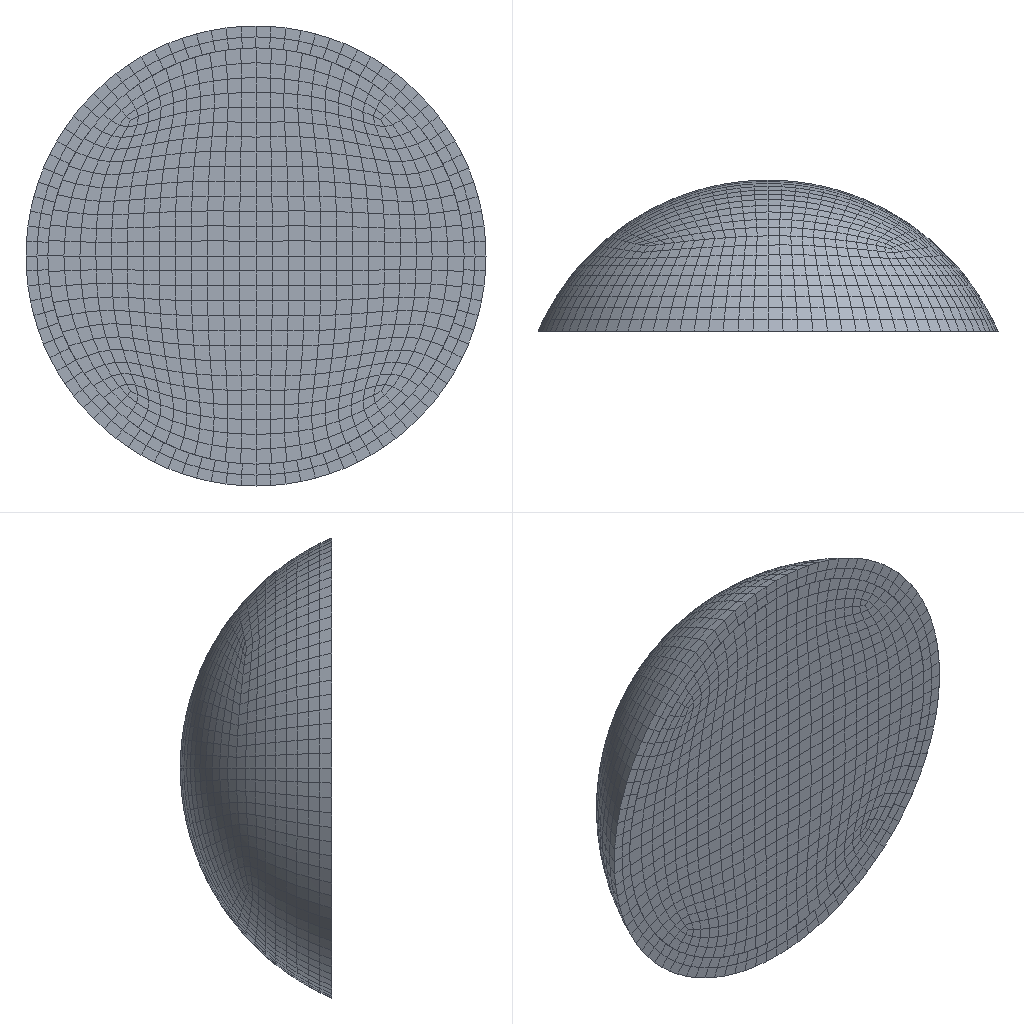Simulation study | abaqus
Set-up summary:
category,name,step,type,value,unit,region
solver,abaqus
solver,version,,,Abaqus/Standard 2020
units,not stated in the deck,,not stated
analysis,deck,,static,static
load_step,Step-1,Step-1,static,nlgeom=True
contact,interactions,,,general=1 pairs=0 ties=0
load_step,requested,,,1
mesh,nodes,,,10810
mesh,elements,,,8352
element_type,C3D8R,,solid,8352
load,load commands in deck,,count,1
bc,support commands in deck,,count,6
material,JITI,,in results
material,MATERIAL-2,,in results
material,MATERIAL-2-COPY,,in results
check,setup vs results,,match,"per instance, exact: element labels, types and connectivity; labels of the nodes the elements use; coordinates not compared"
Abaqus input file, long lists of numbers shortened:
*Heading
** Job name: Job-1 Model name: Model-1
** Generated by: Abaqus/CAE 2020
*Preprint, echo=NO, model=NO, history=NO, contact=NO
**
** PARTS
**
*Part, name=Part-1
*Node
      1,           0.,           0., -0.009499
      2,           0., 0.006,           0.
** (6340 more lines like these left out)
*Element, type=C3D8R
   1,  515,  516, 2283, 2095,   17,   18,  208,  207
   2,  516,  517, 2284, 2283,   18,   19,  209,  208
** (5470 more lines like these left out)
*Node
   6343, 6.44164214e-19, 0.006,           0.
*Nset, nset=Part-1-RefPt_, internal
6343,
*Nset, nset=Set-1, generate
    1,  6342,     1
*Elset, elset=Set-1, generate
    1,  5472,     1
** Section: jiti
*Solid Section, elset=Set-1, material=jiti
,
*End Part
**
*Part, name=mo
*Node
      1,           0., 0.003, 0.007357
      2,           0., 0.003, 0.008609
** (4465 more lines like these left out)
*Element, type=C3D8R
  1,  124,  824, 3248,  594,    1,   19,  548,   66
  2,  824,  130,  709, 3248,   19,    2,   20,  548
** (2878 more lines like these left out)
*Nset, nset=Set-4, generate
    1,  4467,     1
*Elset, elset=Set-4, generate
    1,  2880,     1
*Nset, nset=Set-20
    1,    2,    3,    4,    9,   10,   11,   12,   17,   18,   19,   20,   21,   22,   23,   24
   25,   26,   27,   28,   29,   30,   31,   32,   33,   34,   35,   36,   37,   38,   39,   40
** (170 more lines like these left out)
*Elset, elset=Set-20, generate
  865,  2592,     1
*Nset, nset=Set-21
    1,    2,    3,    4,    5,    6,    7,    8,    9,   10,   11,   12,   13,   14,   15,   16
   19,   20,   21,   22,   23,   24,   25,   26,   27,   28,   29,   30,   31,   32,   33,   34
** (124 more lines like these left out)
*Elset, elset=Set-21
    1,    2,    3,    4,    5,    6,    7,    8,    9,   10,   11,   12,   13,   14,   15,   16
   17,   18,   19,   20,   21,   22,   23,   24,   25,   26,   27,   28,   29,   30,   31,   32
** (70 more lines like these left out)
** Section: mokuai
*Solid Section, elset=Set-21, material=Material-2-Copy
,
** Section: mo
*Solid Section, elset=Set-20, material=Material-2
,
*End Part
**
**
** ASSEMBLY
**
*Assembly, name=Assembly
**
*Instance, name=Part-1-1, part=Part-1
*End Instance
**
*Instance, name=mo-1, part=mo
*End Instance
**
*Nset, nset=Set-3, instance=Part-1-1
 6343,
*Nset, nset=Set-4, instance=mo-1, generate
    1,  4467,     1
*Elset, elset=Set-4, instance=mo-1, generate
    1,  2880,     1
*Nset, nset=Set-5, instance=mo-1, generate
    1,  4467,     1
*Elset, elset=Set-5, instance=mo-1, generate
    1,  2880,     1
*Nset, nset=Set-6, instance=mo-1
 17,
*Nset, nset=Set-7, instance=mo-1
 17,
*Nset, nset=Set-8, instance=mo-1
    5,    6,    7,    8,   13,   14,   15,   16,   17,   18,   67,   68,   69,   70,   71,   72
   73,   74,   75,   76,   77,   78,   79,   80,   81,   82,   83,   84,   85,   86,   87,   88
** (17 more lines like these left out)
*Elset, elset=Set-8, instance=mo-1
  241,  242,  243,  244,  245,  246,  247,  248,  249,  250,  251,  252,  253,  254,  255,  256
  257,  258,  259,  260,  261,  262,  263,  264,  265,  266,  267,  268,  269,  270,  271,  272
** (11 more lines like these left out)
*Nset, nset=Set-9, instance=mo-1, generate
    1,  4467,     1
*Elset, elset=Set-9, instance=mo-1, generate
    1,  2880,     1
*Nset, nset=b_Set-1, instance=Part-1-1, generate
    1,  6342,     1
*Elset, elset=b_Set-1, instance=Part-1-1, generate
    1,  5472,     1
*Nset, nset=_PickedSet7, internal, instance=Part-1-1
 6343,
*Elset, elset=_Surf-1_S1, internal, instance=mo-1, generate
 2737,  2880,     1
*Elset, elset=_Surf-1_S3, internal, instance=mo-1
 1945, 1946, 1947, 1948, 1949, 1950, 1951, 1952, 1953, 1954, 1955, 1956, 1957, 1958, 1959, 1960
 1961, 1962, 1963, 1964, 1965, 1966, 1967, 1968, 1969, 1970, 1971, 1972, 1973, 1974, 1975, 1976
** (21 more lines like these left out)
*Elset, elset=_Surf-1_S4, internal, instance=mo-1
    2,    4,    6,    8,   10,   12,   14,   16,   18,   20,   22,   24,   26,   28,   30,   32
   34,   36,   38,   40,   42,   44,   46,   48,   50,   52,   54,   56,   58,   60,   62,   64
** (21 more lines like these left out)
*Elset, elset=_Surf-1_S5, internal, instance=mo-1
 601, 602, 603, 604, 605, 606, 607, 608, 609, 610, 611, 612, 613, 614, 615, 616
 617, 618, 619, 620, 621, 622, 623, 624, 649, 650, 651, 652, 653, 654, 655, 656
** (7 more lines like these left out)
*Elset, elset=_Surf-1_S2, internal, instance=mo-1
  865,  866,  867,  868,  869,  870,  871,  872,  873,  874,  875,  876,  877,  878,  879,  880
  881,  882,  883,  884,  885,  886,  887,  888,  889,  890,  891,  892,  893,  894,  895,  896
** (25 more lines like these left out)
*Surface, type=ELEMENT, name=Surf-1
_Surf-1_S1, S1
_Surf-1_S3, S3
_Surf-1_S4, S4
_Surf-1_S2, S2
_Surf-1_S5, S5
** Constraint: Constraint-1
*Rigid Body, ref node=_PickedSet7, elset=b_Set-1
*Elset, elset=__Int-1_gcs0_4_S2, internal, instance=Part-1-1
   1,   2,   3,   4,   5,   6,   7,   8,   9,  10,  11,  12,  13,  14,  15,  16
  17,  18,  19,  20,  21,  22,  23,  24,  25,  26,  27,  28,  29,  30,  31,  32
** (13 more lines like these left out)
*Surface, type=ELEMENT, name=_Int-1_gcs0_4, internal
__Int-1_gcs0_4_S2, S2
*Elset, elset=__Int-1_gcs0_5_S4, internal, instance=Part-1-1
 4767, 4770, 4773, 4776, 4779, 4782, 4785, 4788, 4791, 4794, 4797, 4800, 4803, 4806, 4809, 4812
 4815, 4818, 4821, 4824, 4827, 4830, 4833, 4836, 4839, 4842, 4845, 4848, 4851, 4854, 4857, 4860
** (9 more lines like these left out)
*Elset, elset=__Int-1_gcs0_5_S3, internal, instance=Part-1-1
 4945, 4946, 4947, 4948, 4949, 4950, 4951, 4952, 4953, 4954, 4955, 4978, 4979, 4980, 4981, 4982
 4983, 4984, 4985, 4986, 4987, 4988, 5011, 5012, 5013, 5014, 5015, 5016, 5017, 5018, 5019, 5020
** (3 more lines like these left out)
*Surface, type=ELEMENT, name=_Int-1_gcs0_5, internal
__Int-1_gcs0_5_S4, S4
__Int-1_gcs0_5_S3, S3
*Elset, elset=__Int-1_gcs0_10_S3, internal, instance=Part-1-1
 1369, 1370, 1371, 1372, 1373, 1374, 1375, 1376, 1377, 1378, 1399, 1400, 1401, 1402, 1403, 1404
 1405, 1406, 1407, 1408, 1429, 1430, 1431, 1432, 1433, 1434, 1435, 1436, 1437, 1438, 1459, 1460
** (9 more lines like these left out)
*Elset, elset=__Int-1_gcs0_10_S4, internal, instance=Part-1-1, generate
 2211,  2406,     3
*Surface, type=ELEMENT, name=_Int-1_gcs0_10, internal
__Int-1_gcs0_10_S3, S3
__Int-1_gcs0_10_S4, S4
*Elset, elset=__Int-1_gcs0_11_S4, internal, instance=Part-1-1
 2739, 2742, 2745, 2748, 2751, 2754, 2757, 2760, 2763, 2766, 2769, 2772, 2775, 2778, 2781, 2784
 2787, 2790, 2793, 2796, 2799, 2802, 2805, 2808, 2811, 2814, 2817, 2820, 2823, 2826, 2829, 2832
** (9 more lines like these left out)
*Elset, elset=__Int-1_gcs0_11_S3, internal, instance=Part-1-1
 3727, 3728, 3729, 3730, 3731, 3732, 3745, 3746, 3747, 3748, 3749, 3750, 3763, 3764, 3765, 3766
 3767, 3768, 3781, 3782, 3783, 3784, 3785, 3786, 3799, 3800, 3801, 3802, 3803, 3804, 3817, 3818
** (3 more lines like these left out)
*Surface, type=ELEMENT, name=_Int-1_gcs0_11, internal
__Int-1_gcs0_11_S4, S4
__Int-1_gcs0_11_S3, S3
*Elset, elset=__Int-1_gcs0_17_S2, internal, instance=mo-1, generate
  865,  1080,     1
*Surface, type=ELEMENT, name=_Int-1_gcs0_17, internal
__Int-1_gcs0_17_S2, S2
*Elset, elset=__Int-1_gcs0_18_S1, internal, instance=mo-1, generate
 2737,  2880,     1
*Surface, type=ELEMENT, name=_Int-1_gcs0_18, internal
__Int-1_gcs0_18_S1, S1
*Elset, elset=__Int-1_gcs0_20_S6, internal, instance=mo-1, generate
   1,  287,    2
*Surface, type=ELEMENT, name=_Int-1_gcs0_20, internal
__Int-1_gcs0_20_S6, S6
*Elset, elset=__Int-1_gcs0_21_S2, internal, instance=mo-1, generate
 2161,  2376,     1
*Surface, type=ELEMENT, name=_Int-1_gcs0_21, internal
__Int-1_gcs0_21_S2, S2
*Elset, elset=__Int-1_gcs0_23_S3, internal, instance=mo-1
 577, 578, 579, 580, 581, 582, 583, 584, 585, 586, 587, 588, 589, 590, 591, 592
 593, 594, 595, 596, 597, 598, 599, 600, 625, 626, 627, 628, 629, 630, 631, 632
** (7 more lines like these left out)
*Surface, type=ELEMENT, name=_Int-1_gcs0_23, internal
__Int-1_gcs0_23_S3, S3
*Elset, elset=__Int-1_gcs0_25_S4, internal, instance=mo-1, generate
 290,  576,    2
*Surface, type=ELEMENT, name=_Int-1_gcs0_25, internal
__Int-1_gcs0_25_S4, S4
*Elset, elset=__Int-1_gcs0_26_S3, internal, instance=mo-1
 1945, 1946, 1947, 1948, 1949, 1950, 1951, 1952, 1953, 1954, 1955, 1956, 1957, 1958, 1959, 1960
 1961, 1962, 1963, 1964, 1965, 1966, 1967, 1968, 1969, 1970, 1971, 1972, 1973, 1974, 1975, 1976
** (10 more lines like these left out)
*Elset, elset=__Int-1_gcs0_26_S4, internal, instance=mo-1, generate
 1981,  2016,     1
*Surface, type=ELEMENT, name=_Int-1_gcs0_26, internal
__Int-1_gcs0_26_S3, S3
__Int-1_gcs0_26_S4, S4
*Elset, elset=__Int-1_gcs0_27_S3, internal, instance=mo-1, generate
 1513,  1548,     1
*Elset, elset=__Int-1_gcs0_27_S4, internal, instance=mo-1, generate
 1549,  1728,     1
*Surface, type=ELEMENT, name=_Int-1_gcs0_27, internal
__Int-1_gcs0_27_S3, S3
__Int-1_gcs0_27_S4, S4
*Elset, elset=__Int-1_gcs0_32_S3, internal, instance=mo-1
 2377, 2378, 2379, 2380, 2381, 2382, 2383, 2384, 2385, 2386, 2387, 2388, 2389, 2390, 2391, 2392
 2393, 2394, 2395, 2396, 2397, 2398, 2399, 2400, 2401, 2402, 2403, 2404, 2405, 2406, 2407, 2408
** (10 more lines like these left out)
*Elset, elset=__Int-1_gcs0_32_S4, internal, instance=mo-1, generate
 2413,  2448,     1
*Surface, type=ELEMENT, name=_Int-1_gcs0_32, internal
__Int-1_gcs0_32_S3, S3
__Int-1_gcs0_32_S4, S4
*Elset, elset=__Int-1_gcs0_34_S6, internal, instance=mo-1, generate
 289,  575,    2
*Surface, type=ELEMENT, name=_Int-1_gcs0_34, internal
__Int-1_gcs0_34_S6, S6
*Elset, elset=__Int-1_gcs0_35_S3, internal, instance=mo-1, generate
 1081,  1116,     1
*Elset, elset=__Int-1_gcs0_35_S4, internal, instance=mo-1, generate
 1117,  1296,     1
*Surface, type=ELEMENT, name=_Int-1_gcs0_35, internal
__Int-1_gcs0_35_S3, S3
__Int-1_gcs0_35_S4, S4
*Elset, elset=__Int-1_gcs0_36_S5, internal, instance=mo-1
 601, 602, 603, 604, 605, 606, 607, 608, 609, 610, 611, 612, 613, 614, 615, 616
 617, 618, 619, 620, 621, 622, 623, 624, 649, 650, 651, 652, 653, 654, 655, 656
** (7 more lines like these left out)
*Surface, type=ELEMENT, name=_Int-1_gcs0_36, internal
__Int-1_gcs0_36_S5, S5
*Elset, elset=__Int-1_gcs0_39_S2, internal, instance=mo-1, generate
 1729,  1944,     1
*Surface, type=ELEMENT, name=_Int-1_gcs0_39, internal
__Int-1_gcs0_39_S2, S2
*Elset, elset=__Int-1_gcs0_41_S2, internal, instance=mo-1, generate
 1297,  1512,     1
*Surface, type=ELEMENT, name=_Int-1_gcs0_41, internal
__Int-1_gcs0_41_S2, S2
*Elset, elset=__Int-1_gcs0_42_S4, internal, instance=mo-1, generate
   2,  288,    2
*Surface, type=ELEMENT, name=_Int-1_gcs0_42, internal
__Int-1_gcs0_42_S4, S4
*Elset, elset=__Int-1_gcs0_44_S2, internal, instance=mo-1, generate
 2593,  2736,     1
*Surface, type=ELEMENT, name=_Int-1_gcs0_44, internal
__Int-1_gcs0_44_S2, S2
*End Assembly
*Amplitude, name=Amp-1
             0.,              0.,              1.,              1.
**
** MATERIALS
**
*Material, name=Material-2
*Density
 1.1e-09,
*Elastic
1., 0.4
*Expansion
 -0.001,
*Material, name=Material-2-Copy
*Density
 1.1e-09,
*Elastic
1., 0.4
*Expansion
 -0.0011,
*Material, name=jiti
*Density
 7.8e-09,
*Elastic
210000., 0.3
**
** INTERACTION PROPERTIES
**
*Surface Interaction, name=IntProp-1
1.,
*Friction, slip tolerance=0.005
 0.15,
*Surface Behavior, pressure-overclosure=HARD
**
** PREDEFINED FIELDS
**
** Name: Predefined Field-1   Type: Temperature
*Initial Conditions, type=TEMPERATURE
Set-4, 20.
**
** INTERACTIONS
**
** Interaction: Int-1
*Contact
*Contact Inclusions, ALL EXTERIOR
*Contact Property Assignment
 ,  , IntProp-1
*Surface Property Assignment, property=GEOMETRIC CORRECTION
_Int-1_gcs0_4, Spherical, 0., -0.00452, 0.
_Int-1_gcs0_5, Spherical, 0., -0.00452, 0.
_Int-1_gcs0_10, Spherical, 0., -0.00452, 0.
_Int-1_gcs0_11, Spherical, 0., -0.00452, 0.
_Int-1_gcs0_17, Spherical, 0., -0.00452, 0.
_Int-1_gcs0_18, Spherical, 0., -0.00452, 0.
_Int-1_gcs0_20, Spherical, 0., -0.00452, 0.
_Int-1_gcs0_21, Spherical, 0., -0.00452, 0.
_Int-1_gcs0_23, Spherical, 0., -0.00452, 0.
_Int-1_gcs0_25, Spherical, 0., -0.00452, 0.
_Int-1_gcs0_26, Spherical, 0., -0.00452, 0.
_Int-1_gcs0_27, Spherical, 0., -0.00452, 0.
_Int-1_gcs0_32, Spherical, 0., -0.00452, 0.
_Int-1_gcs0_34, Spherical, 0., -0.00452, 0.
_Int-1_gcs0_35, Spherical, 0., -0.00452, 0.
_Int-1_gcs0_36, Spherical, 0., -0.00452, 0.
_Int-1_gcs0_39, Spherical, 0., -0.00452, 0.
_Int-1_gcs0_41, Spherical, 0., -0.00452, 0.
_Int-1_gcs0_42, Spherical, 0., -0.00452, 0.
_Int-1_gcs0_44, Spherical, 0., -0.00452, 0.
** ----------------------------------------------------------------
**
** STEP: Step-1
**
*Step, name=Step-1, nlgeom=YES, inc=1000
*Static, stabilize=0.0002, allsdtol=0.05, continue=NO
0.01, 1., 1e-05, 1.
**
** BOUNDARY CONDITIONS
**
** Name: BC-1 Type: 对称/反对称/完全固定
*Boundary
Set-3, ENCASTRE
** Name: BC-2 Type: 位移/转角
*Boundary, amplitude=Amp-1
Set-7, 1, 1
Set-7, 3, 3
Set-7, 4, 4
Set-7, 5, 5
Set-7, 6, 6
**
** PREDEFINED FIELDS
**
** Name: Predefined Field-2   Type: Temperature
*Temperature, amplitude=Amp-1
Set-9, 800.
**
** OUTPUT REQUESTS
**
*Restart, write, number interval=1, time marks=NO
**
** FIELD OUTPUT: F-Output-1
**
*Output, field
*Node Output
CF, RF, RM, RT, U, V
*Element Output, directions=YES
E, LE, MISES, PE, PEEQ, S, SF
*Contact Output
CDISP, CFORCE, CSTRESS
**
** HISTORY OUTPUT: H-Output-1
**
*Output, history, variable=PRESELECT
*End Step
Results summary:
result,step,,completed,increments=21 time=1.0/1.0
result,analysis,,,static
result,last_loadstep,,,1
result,analysis steps,,count,1
result,primary field,,,U
result,reaction total,,FX,0.0,model units
result,reaction total,,FY,0.0,model units
result,reaction total,,FZ,0.0,model units